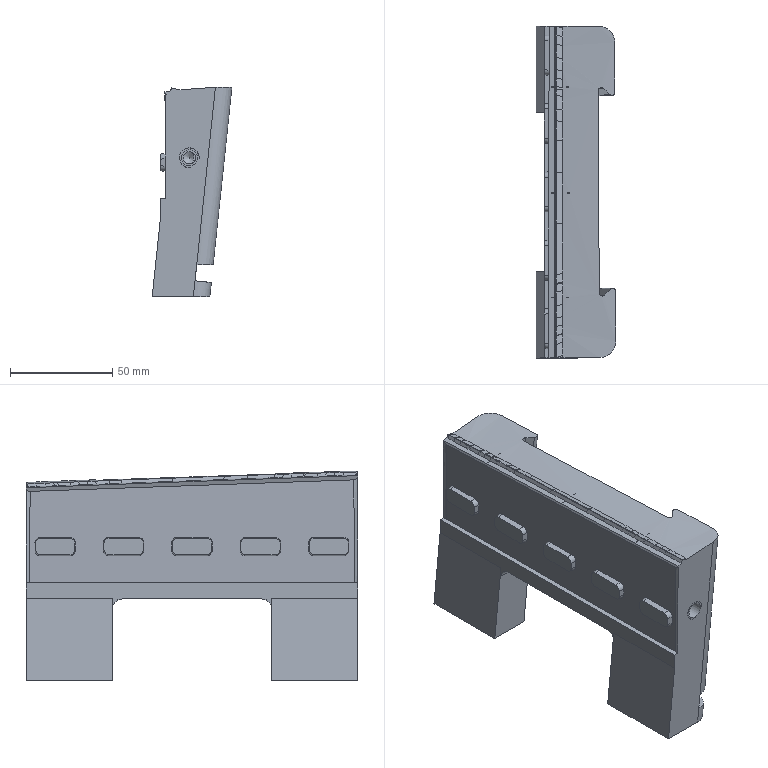Part | STEP file | P011002L001-000 | 1 solid | 315 faces | box 38.903 x 161.923 x 102.441 mm | volume 296499 mm3 | plane 144 | spline 67 | cylinder 48 | other 29 | cone 27 | commonest cylinder face diameters 5 x20 3 x10 16 x6 6 x3 2.5 x2 2.99 x2